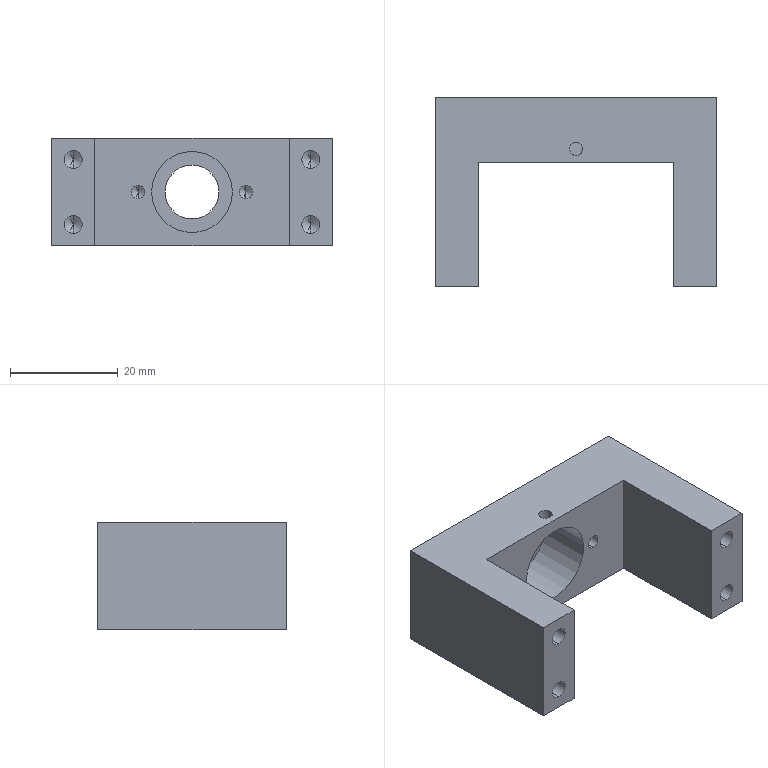Part | SolidWorks | features HoleWzd 3, ICE 3, Extrusion 1 | 1 solid | 41 faces | box 52 x 35 x 20 mm | volume 17449 mm3 | cylinder 18 | cone 12 | plane 11 | commonest cylinder face diameters 3.3 x8 2.5 x6 10 x2 15 x2
STEP:
#1=CARTESIAN_POINT('',(-10.,26.259,1.25));
#2=VERTEX_POINT('',#1);
#3=CARTESIAN_POINT('',(-10.,26.259,-1.25));
#4=VERTEX_POINT('',#3);
#5=CARTESIAN_POINT('',(-10.,26.259,0.));
#6=DIRECTION('',(0.,-1.,0.));
#7=DIRECTION('',(0.,0.,-1.));
#8=AXIS2_PLACEMENT_3D('',#5,#6,#7);
#9=CIRCLE('',#8,1.25);
#10=EDGE_CURVE('',#2,#4,#9,.T.);
#11=ORIENTED_EDGE('',*,*,#10,.F.);
#12=CARTESIAN_POINT('',(-10.,16.259,1.25));
#13=VERTEX_POINT('',#12);
#14=CARTESIAN_POINT('',(-10.,16.259,1.25));
#15=DIRECTION('',(0.,-1.,0.));
#16=VECTOR('',#15,1000.);
#17=LINE('',#14,#16);
#18=EDGE_CURVE('',#2,#13,#17,.T.);
#19=ORIENTED_EDGE('',*,*,#18,.T.);
#20=CARTESIAN_POINT('',(-10.,16.259,-1.25));
#21=VERTEX_POINT('',#20);
#22=CARTESIAN_POINT('',(-10.,16.259,0.));
#23=DIRECTION('',(0.,-1.,0.));
#24=DIRECTION('',(0.,0.,-1.));
#25=AXIS2_PLACEMENT_3D('',#22,#23,#24);
#26=CIRCLE('',#25,1.25);
#27=EDGE_CURVE('',#13,#21,#26,.T.);
#28=ORIENTED_EDGE('',*,*,#27,.T.);
#29=CARTESIAN_POINT('',(-10.,16.259,-1.25));
#30=DIRECTION('',(0.,-1.,0.));
#31=VECTOR('',#30,1000.);
#32=LINE('',#29,#31);
#33=EDGE_CURVE('',#4,#21,#32,.T.);
#34=ORIENTED_EDGE('',*,*,#33,.F.);
#35=EDGE_LOOP('',(#11,#19,#28,#34));
#36=FACE_OUTER_BOUND('',#35,.T.);
#37=CARTESIAN_POINT('',(-10.,16.259,0.));
#38=DIRECTION('',(0.,-1.,0.));
#39=DIRECTION('',(0.,0.,-1.));
#40=AXIS2_PLACEMENT_3D('',#37,#38,#39);
#41=CYLINDRICAL_SURFACE('',#40,1.25);
#42=ADVANCED_FACE('',(#36),#41,.F.);
#43=CARTESIAN_POINT('',(-10.,27.01,0.));
#44=VERTEX_POINT('',#43);
#45=CARTESIAN_POINT('',(-10.,26.259,-1.25));
#46=DIRECTION('',(0.,-0.515,-0.8572));
#47=VECTOR('',#46,1000.);
#48=LINE('',#45,#47);
#49=EDGE_CURVE('',#44,#4,#48,.T.);
#50=ORIENTED_EDGE('',*,*,#49,.F.);
#51=CARTESIAN_POINT('',(-10.,26.259,1.25));
#52=DIRECTION('',(0.,-0.515,0.8572));
#53=VECTOR('',#52,1000.);
#54=LINE('',#51,#53);
#55=EDGE_CURVE('',#44,#2,#54,.T.);
#56=ORIENTED_EDGE('',*,*,#55,.T.);
#57=ORIENTED_EDGE('',*,*,#10,.T.);
#58=EDGE_LOOP('',(#50,#56,#57));
#59=FACE_OUTER_BOUND('',#58,.T.);
#60=CARTESIAN_POINT('',(-10.,26.259,0.));
#61=DIRECTION('',(0.,-1.,0.));
#62=DIRECTION('',(0.,0.,-1.));
#63=AXIS2_PLACEMENT_3D('',#60,#61,#62);
#64=CONICAL_SURFACE('',#63,1.25,1.03);
#65=ADVANCED_FACE('',(#59),#64,.F.);
#66=CARTESIAN_POINT('',(10.,26.259,1.25));
#67=VERTEX_POINT('',#66);
#68=CARTESIAN_POINT('',(10.,26.259,-1.25));
#69=VERTEX_POINT('',#68);
#70=CARTESIAN_POINT('',(10.,26.259,0.));
#71=DIRECTION('',(0.,-1.,0.));
#72=DIRECTION('',(0.,0.,-1.));
#73=AXIS2_PLACEMENT_3D('',#70,#71,#72);
#74=CIRCLE('',#73,1.25);
#75=EDGE_CURVE('',#67,#69,#74,.T.);
#76=ORIENTED_EDGE('',*,*,#75,.F.);
#77=CARTESIAN_POINT('',(10.,16.259,1.25));
#78=VERTEX_POINT('',#77);
#79=CARTESIAN_POINT('',(10.,16.259,1.25));
#80=DIRECTION('',(0.,-1.,0.));
#81=VECTOR('',#80,1000.);
#82=LINE('',#79,#81);
#83=EDGE_CURVE('',#67,#78,#82,.T.);
#84=ORIENTED_EDGE('',*,*,#83,.T.);
#85=CARTESIAN_POINT('',(10.,16.259,-1.25));
#86=VERTEX_POINT('',#85);
#87=CARTESIAN_POINT('',(10.,16.259,0.));
#88=DIRECTION('',(0.,-1.,0.));
#89=DIRECTION('',(0.,0.,-1.));
#90=AXIS2_PLACEMENT_3D('',#87,#88,#89);
#91=CIRCLE('',#90,1.25);
#92=EDGE_CURVE('',#78,#86,#91,.T.);
#93=ORIENTED_EDGE('',*,*,#92,.T.);
#94=CARTESIAN_POINT('',(10.,16.259,-1.25));
#95=DIRECTION('',(0.,-1.,0.));
#96=VECTOR('',#95,1000.);
#97=LINE('',#94,#96);
#98=EDGE_CURVE('',#69,#86,#97,.T.);
#99=ORIENTED_EDGE('',*,*,#98,.F.);
#100=EDGE_LOOP('',(#76,#84,#93,#99));
#101=FACE_OUTER_BOUND('',#100,.T.);
#102=CARTESIAN_POINT('',(10.,16.259,0.));
#103=DIRECTION('',(0.,-1.,0.));
#104=DIRECTION('',(0.,0.,-1.));
#105=AXIS2_PLACEMENT_3D('',#102,#103,#104);
#106=CYLINDRICAL_SURFACE('',#105,1.25);
#107=ADVANCED_FACE('',(#101),#106,.F.);
#108=CARTESIAN_POINT('',(10.,27.01,0.));
#109=VERTEX_POINT('',#108);
#110=CARTESIAN_POINT('',(10.,26.259,-1.25));
#111=DIRECTION('',(0.,-0.515,-0.8572));
#112=VECTOR('',#111,1000.);
#113=LINE('',#110,#112);
#114=EDGE_CURVE('',#109,#69,#113,.T.);
#115=ORIENTED_EDGE('',*,*,#114,.F.);
#116=CARTESIAN_POINT('',(10.,26.259,1.25));
#117=DIRECTION('',(0.,-0.515,0.8572));
#118=VECTOR('',#117,1000.);
#119=LINE('',#116,#118);
#120=EDGE_CURVE('',#109,#67,#119,.T.);
#121=ORIENTED_EDGE('',*,*,#120,.T.);
#122=ORIENTED_EDGE('',*,*,#75,.T.);
#123=EDGE_LOOP('',(#115,#121,#122));
#124=FACE_OUTER_BOUND('',#123,.T.);
#125=CARTESIAN_POINT('',(10.,26.259,0.));
#126=DIRECTION('',(0.,-1.,0.));
#127=DIRECTION('',(0.,0.,-1.));
#128=AXIS2_PLACEMENT_3D('',#125,#126,#127);
#129=CONICAL_SURFACE('',#128,1.25,1.03);
#130=ADVANCED_FACE('',(#124),#129,.F.);
#131=CARTESIAN_POINT('',(-1.25,18.759,7.395));
#132=VERTEX_POINT('',#131);
#133=CARTESIAN_POINT('',(1.25,18.759,7.395));
#134=VERTEX_POINT('',#133);
#135=CARTESIAN_POINT('',(-1.25,18.759,7.395));
#136=CARTESIAN_POINT('',(-1.25,18.596,7.395));
#137=CARTESIAN_POINT('',(-1.217,18.431,7.401));
#138=CARTESIAN_POINT('',(-1.092,18.13,7.42));
#139=CARTESIAN_POINT('',(-0.9996,17.991,7.434));
#140=CARTESIAN_POINT('',(-0.8269,17.818,7.455));
#141=CARTESIAN_POINT('',(-0.7627,17.766,7.461));
#142=CARTESIAN_POINT('',(-0.6272,17.675,7.474));
#143=CARTESIAN_POINT('',(-0.5555,17.636,7.48));
#144=CARTESIAN_POINT('',(-0.3283,17.542,7.494));
#145=CARTESIAN_POINT('',(-0.1659,17.509,7.5));
#146=CARTESIAN_POINT('',(0.1644,17.509,7.5));
#147=CARTESIAN_POINT('',(0.3271,17.542,7.494));
#148=CARTESIAN_POINT('',(0.6295,17.667,7.475));
#149=CARTESIAN_POINT('',(0.7682,17.76,7.461));
#150=CARTESIAN_POINT('',(0.9984,17.99,7.434));
#151=CARTESIAN_POINT('',(1.092,18.129,7.42));
#152=CARTESIAN_POINT('',(1.217,18.429,7.401));
#153=CARTESIAN_POINT('',(1.25,18.594,7.395));
#154=CARTESIAN_POINT('',(1.25,18.759,7.395));
#155=B_SPLINE_CURVE_WITH_KNOTS('',3,(#135,#136,#137,#138,#139,#140,#141,#142,#143,#144,#145,#146,#147,#148,#149,#150,#151,#152,#153,#154),.UNSPECIFIED.,.F.,.F.,(4,2,2,2,2,2,2,2,2,4),(0.003915,0.004404,0.004893,0.005138,0.005383,0.005872,0.006361,0.00685,0.00734,0.007829),.UNSPECIFIED.);
#156=EDGE_CURVE('',#132,#134,#155,.T.);
#157=ORIENTED_EDGE('',*,*,#156,.F.);
#158=CARTESIAN_POINT('',(-1.25,18.759,10.));
#159=VERTEX_POINT('',#158);
#160=CARTESIAN_POINT('',(-1.25,18.759,10.));
#161=DIRECTION('',(0.,0.,1.));
#162=VECTOR('',#161,1000.);
#163=LINE('',#160,#162);
#164=EDGE_CURVE('',#132,#159,#163,.T.);
#165=ORIENTED_EDGE('',*,*,#164,.T.);
#166=CARTESIAN_POINT('',(1.25,18.759,10.));
#167=VERTEX_POINT('',#166);
#168=CARTESIAN_POINT('',(0.,18.759,10.));
#169=DIRECTION('',(0.,0.,1.));
#170=DIRECTION('',(1.,0.,0.));
#171=AXIS2_PLACEMENT_3D('',#168,#169,#170);
#172=CIRCLE('',#171,1.25);
#173=EDGE_CURVE('',#159,#167,#172,.T.);
#174=ORIENTED_EDGE('',*,*,#173,.T.);
#175=CARTESIAN_POINT('',(1.25,18.759,10.));
#176=DIRECTION('',(0.,0.,1.));
#177=VECTOR('',#176,1000.);
#178=LINE('',#175,#177);
#179=EDGE_CURVE('',#134,#167,#178,.T.);
#180=ORIENTED_EDGE('',*,*,#179,.F.);
#181=EDGE_LOOP('',(#157,#165,#174,#180));
#182=FACE_OUTER_BOUND('',#181,.T.);
#183=CARTESIAN_POINT('',(0.,18.759,10.));
#184=DIRECTION('',(0.,0.,1.));
#185=DIRECTION('',(1.,0.,0.));
#186=AXIS2_PLACEMENT_3D('',#183,#184,#185);
#187=CYLINDRICAL_SURFACE('',#186,1.25);
#188=ADVANCED_FACE('',(#182),#187,.F.);
#189=CARTESIAN_POINT('',(-7.5,26.259,0.));
#190=VERTEX_POINT('',#189);
#191=CARTESIAN_POINT('',(7.5,26.259,0.));
#192=VERTEX_POINT('',#191);
#193=CARTESIAN_POINT('',(0.,26.259,0.));
#194=DIRECTION('',(0.,-1.,0.));
#195=DIRECTION('',(1.,0.,0.));
#196=AXIS2_PLACEMENT_3D('',#193,#194,#195);
#197=CIRCLE('',#196,7.5);
#198=EDGE_CURVE('',#190,#192,#197,.T.);
#199=ORIENTED_EDGE('',*,*,#198,.F.);
#200=CARTESIAN_POINT('',(-7.5,16.259,0.));
#201=VERTEX_POINT('',#200);
#202=CARTESIAN_POINT('',(-7.5,26.259,0.));
#203=DIRECTION('',(0.,-1.,0.));
#204=VECTOR('',#203,1000.);
#205=LINE('',#202,#204);
#206=EDGE_CURVE('',#190,#201,#205,.T.);
#207=ORIENTED_EDGE('',*,*,#206,.T.);
#208=CARTESIAN_POINT('',(7.5,16.259,0.));
#209=VERTEX_POINT('',#208);
#210=CARTESIAN_POINT('',(0.,16.259,0.));
#211=DIRECTION('',(0.,-1.,0.));
#212=DIRECTION('',(1.,0.,0.));
#213=AXIS2_PLACEMENT_3D('',#210,#211,#212);
#214=CIRCLE('',#213,7.5);
#215=EDGE_CURVE('',#201,#209,#214,.T.);
#216=ORIENTED_EDGE('',*,*,#215,.T.);
#217=CARTESIAN_POINT('',(7.5,26.259,0.));
#218=DIRECTION('',(0.,-1.,0.));
#219=VECTOR('',#218,1000.);
#220=LINE('',#217,#219);
#221=EDGE_CURVE('',#192,#209,#220,.T.);
#222=ORIENTED_EDGE('',*,*,#221,.F.);
#223=EDGE_LOOP('',(#199,#207,#216,#222));
#224=FACE_OUTER_BOUND('',#223,.T.);
#225=CARTESIAN_POINT('',(0.,26.259,0.));
#226=DIRECTION('',(0.,-1.,0.));
#227=DIRECTION('',(1.,0.,0.));
#228=AXIS2_PLACEMENT_3D('',#225,#226,#227);
#229=CYLINDRICAL_SURFACE('',#228,7.5);
#230=ADVANCED_FACE('',(#224),#229,.F.);
#231=CARTESIAN_POINT('',(22.,3.259,-4.35));
#232=VERTEX_POINT('',#231);
#233=CARTESIAN_POINT('',(22.,3.259,-7.65));
#234=VERTEX_POINT('',#233);
#235=CARTESIAN_POINT('',(22.,3.259,-6.));
#236=DIRECTION('',(0.,-1.,0.));
#237=DIRECTION('',(0.,0.,-1.));
#238=AXIS2_PLACEMENT_3D('',#235,#236,#237);
#239=CIRCLE('',#238,1.65);
#240=EDGE_CURVE('',#232,#234,#239,.T.);
#241=ORIENTED_EDGE('',*,*,#240,.F.);
#242=CARTESIAN_POINT('',(22.,-6.741,-4.35));
#243=VERTEX_POINT('',#242);
#244=CARTESIAN_POINT('',(22.,-6.741,-4.35));
#245=DIRECTION('',(0.,-1.,0.));
#246=VECTOR('',#245,1000.);
#247=LINE('',#244,#246);
#248=EDGE_CURVE('',#232,#243,#247,.T.);
#249=ORIENTED_EDGE('',*,*,#248,.T.);
#250=CARTESIAN_POINT('',(22.,-6.741,-7.65));
#251=VERTEX_POINT('',#250);
#252=CARTESIAN_POINT('',(22.,-6.741,-6.));
#253=DIRECTION('',(0.,-1.,0.));
#254=DIRECTION('',(0.,0.,-1.));
#255=AXIS2_PLACEMENT_3D('',#252,#253,#254);
#256=CIRCLE('',#255,1.65);
#257=EDGE_CURVE('',#243,#251,#256,.T.);
#258=ORIENTED_EDGE('',*,*,#257,.T.);
#259=CARTESIAN_POINT('',(22.,-6.741,-7.65));
#260=DIRECTION('',(0.,-1.,0.));
#261=VECTOR('',#260,1000.);
#262=LINE('',#259,#261);
#263=EDGE_CURVE('',#234,#251,#262,.T.);
#264=ORIENTED_EDGE('',*,*,#263,.F.);
#265=EDGE_LOOP('',(#241,#249,#258,#264));
#266=FACE_OUTER_BOUND('',#265,.T.);
#267=CARTESIAN_POINT('',(22.,-6.741,-6.));
#268=DIRECTION('',(0.,-1.,0.));
#269=DIRECTION('',(0.,0.,-1.));
#270=AXIS2_PLACEMENT_3D('',#267,#268,#269);
#271=CYLINDRICAL_SURFACE('',#270,1.65);
#272=ADVANCED_FACE('',(#266),#271,.F.);
#273=CARTESIAN_POINT('',(22.,4.251,-6.));
#274=VERTEX_POINT('',#273);
#275=CARTESIAN_POINT('',(22.,3.259,-7.65));
#276=DIRECTION('',(0.,-0.515,-0.8572));
#277=VECTOR('',#276,1000.);
#278=LINE('',#275,#277);
#279=EDGE_CURVE('',#274,#234,#278,.T.);
#280=ORIENTED_EDGE('',*,*,#279,.F.);
#281=CARTESIAN_POINT('',(22.,3.259,-4.35));
#282=DIRECTION('',(0.,-0.515,0.8572));
#283=VECTOR('',#282,1000.);
#284=LINE('',#281,#283);
#285=EDGE_CURVE('',#274,#232,#284,.T.);
#286=ORIENTED_EDGE('',*,*,#285,.T.);
#287=ORIENTED_EDGE('',*,*,#240,.T.);
#288=EDGE_LOOP('',(#280,#286,#287));
#289=FACE_OUTER_BOUND('',#288,.T.);
#290=CARTESIAN_POINT('',(22.,3.259,-6.));
#291=DIRECTION('',(0.,-1.,0.));
#292=DIRECTION('',(0.,0.,-1.));
#293=AXIS2_PLACEMENT_3D('',#290,#291,#292);
#294=CONICAL_SURFACE('',#293,1.65,1.03);
#295=ADVANCED_FACE('',(#289),#294,.F.);
#296=CARTESIAN_POINT('',(22.,3.259,7.65));
#297=VERTEX_POINT('',#296);
#298=CARTESIAN_POINT('',(22.,3.259,4.35));
#299=VERTEX_POINT('',#298);
#300=CARTESIAN_POINT('',(22.,3.259,6.));
#301=DIRECTION('',(0.,-1.,0.));
#302=DIRECTION('',(0.,0.,-1.));
#303=AXIS2_PLACEMENT_3D('',#300,#301,#302);
#304=CIRCLE('',#303,1.65);
#305=EDGE_CURVE('',#297,#299,#304,.T.);
#306=ORIENTED_EDGE('',*,*,#305,.F.);
#307=CARTESIAN_POINT('',(22.,-6.741,7.65));
#308=VERTEX_POINT('',#307);
#309=CARTESIAN_POINT('',(22.,-6.741,7.65));
#310=DIRECTION('',(0.,-1.,0.));
#311=VECTOR('',#310,1000.);
#312=LINE('',#309,#311);
#313=EDGE_CURVE('',#297,#308,#312,.T.);
#314=ORIENTED_EDGE('',*,*,#313,.T.);
#315=CARTESIAN_POINT('',(22.,-6.741,4.35));
#316=VERTEX_POINT('',#315);
#317=CARTESIAN_POINT('',(22.,-6.741,6.));
#318=DIRECTION('',(0.,-1.,0.));
#319=DIRECTION('',(0.,0.,-1.));
#320=AXIS2_PLACEMENT_3D('',#317,#318,#319);
#321=CIRCLE('',#320,1.65);
#322=EDGE_CURVE('',#308,#316,#321,.T.);
#323=ORIENTED_EDGE('',*,*,#322,.T.);
#324=CARTESIAN_POINT('',(22.,-6.741,4.35));
#325=DIRECTION('',(0.,-1.,0.));
#326=VECTOR('',#325,1000.);
#327=LINE('',#324,#326);
#328=EDGE_CURVE('',#299,#316,#327,.T.);
#329=ORIENTED_EDGE('',*,*,#328,.F.);
#330=EDGE_LOOP('',(#306,#314,#323,#329));
#331=FACE_OUTER_BOUND('',#330,.T.);
#332=CARTESIAN_POINT('',(22.,-6.741,6.));
#333=DIRECTION('',(0.,-1.,0.));
#334=DIRECTION('',(0.,0.,-1.));
#335=AXIS2_PLACEMENT_3D('',#332,#333,#334);
#336=CYLINDRICAL_SURFACE('',#335,1.65);
#337=ADVANCED_FACE('',(#331),#336,.F.);
#338=CARTESIAN_POINT('',(22.,4.251,6.));
#339=VERTEX_POINT('',#338);
#340=CARTESIAN_POINT('',(22.,3.259,4.35));
#341=DIRECTION('',(0.,-0.515,-0.8572));
#342=VECTOR('',#341,1000.);
#343=LINE('',#340,#342);
#344=EDGE_CURVE('',#339,#299,#343,.T.);
#345=ORIENTED_EDGE('',*,*,#344,.F.);
#346=CARTESIAN_POINT('',(22.,3.259,7.65));
#347=DIRECTION('',(0.,-0.515,0.8572));
#348=VECTOR('',#347,1000.);
#349=LINE('',#346,#348);
#350=EDGE_CURVE('',#339,#297,#349,.T.);
#351=ORIENTED_EDGE('',*,*,#350,.T.);
#352=ORIENTED_EDGE('',*,*,#305,.T.);
#353=EDGE_LOOP('',(#345,#351,#352));
#354=FACE_OUTER_BOUND('',#353,.T.);
#355=CARTESIAN_POINT('',(22.,3.259,6.));
#356=DIRECTION('',(0.,-1.,0.));
#357=DIRECTION('',(0.,0.,-1.));
#358=AXIS2_PLACEMENT_3D('',#355,#356,#357);
#359=CONICAL_SURFACE('',#358,1.65,1.03);
#360=ADVANCED_FACE('',(#354),#359,.F.);
#361=CARTESIAN_POINT('',(-22.,3.259,-4.35));
#362=VERTEX_POINT('',#361);
#363=CARTESIAN_POINT('',(-22.,3.259,-7.65));
#364=VERTEX_POINT('',#363);
#365=CARTESIAN_POINT('',(-22.,3.259,-6.));
#366=DIRECTION('',(0.,-1.,0.));
#367=DIRECTION('',(0.,0.,-1.));
#368=AXIS2_PLACEMENT_3D('',#365,#366,#367);
#369=CIRCLE('',#368,1.65);
#370=EDGE_CURVE('',#362,#364,#369,.T.);
#371=ORIENTED_EDGE('',*,*,#370,.F.);
#372=CARTESIAN_POINT('',(-22.,-6.741,-4.35));
#373=VERTEX_POINT('',#372);
#374=CARTESIAN_POINT('',(-22.,-6.741,-4.35));
#375=DIRECTION('',(0.,-1.,0.));
#376=VECTOR('',#375,1000.);
#377=LINE('',#374,#376);
#378=EDGE_CURVE('',#362,#373,#377,.T.);
#379=ORIENTED_EDGE('',*,*,#378,.T.);
#380=CARTESIAN_POINT('',(-22.,-6.741,-7.65));
#381=VERTEX_POINT('',#380);
#382=CARTESIAN_POINT('',(-22.,-6.741,-6.));
#383=DIRECTION('',(0.,-1.,0.));
#384=DIRECTION('',(0.,0.,-1.));
#385=AXIS2_PLACEMENT_3D('',#382,#383,#384);
#386=CIRCLE('',#385,1.65);
#387=EDGE_CURVE('',#373,#381,#386,.T.);
#388=ORIENTED_EDGE('',*,*,#387,.T.);
#389=CARTESIAN_POINT('',(-22.,-6.741,-7.65));
#390=DIRECTION('',(0.,-1.,0.));
#391=VECTOR('',#390,1000.);
#392=LINE('',#389,#391);
#393=EDGE_CURVE('',#364,#381,#392,.T.);
#394=ORIENTED_EDGE('',*,*,#393,.F.);
#395=EDGE_LOOP('',(#371,#379,#388,#394));
#396=FACE_OUTER_BOUND('',#395,.T.);
#397=CARTESIAN_POINT('',(-22.,-6.741,-6.));
#398=DIRECTION('',(0.,-1.,0.));
#399=DIRECTION('',(0.,0.,-1.));
#400=AXIS2_PLACEMENT_3D('',#397,#398,#399);
#401=CYLINDRICAL_SURFACE('',#400,1.65);
#402=ADVANCED_FACE('',(#396),#401,.F.);
#403=CARTESIAN_POINT('',(-22.,4.251,-6.));
#404=VERTEX_POINT('',#403);
#405=CARTESIAN_POINT('',(-22.,3.259,-7.65));
#406=DIRECTION('',(0.,-0.515,-0.8572));
#407=VECTOR('',#406,1000.);
#408=LINE('',#405,#407);
#409=EDGE_CURVE('',#404,#364,#408,.T.);
#410=ORIENTED_EDGE('',*,*,#409,.F.);
#411=CARTESIAN_POINT('',(-22.,3.259,-4.35));
#412=DIRECTION('',(0.,-0.515,0.8572));
#413=VECTOR('',#412,1000.);
#414=LINE('',#411,#413);
#415=EDGE_CURVE('',#404,#362,#414,.T.);
#416=ORIENTED_EDGE('',*,*,#415,.T.);
#417=ORIENTED_EDGE('',*,*,#370,.T.);
#418=EDGE_LOOP('',(#410,#416,#417));
#419=FACE_OUTER_BOUND('',#418,.T.);
#420=CARTESIAN_POINT('',(-22.,3.259,-6.));
#421=DIRECTION('',(0.,-1.,0.));
#422=DIRECTION('',(0.,0.,-1.));
#423=AXIS2_PLACEMENT_3D('',#420,#421,#422);
#424=CONICAL_SURFACE('',#423,1.65,1.03);
#425=ADVANCED_FACE('',(#419),#424,.F.);
#426=CARTESIAN_POINT('',(-22.,3.259,7.65));
#427=VERTEX_POINT('',#426);
#428=CARTESIAN_POINT('',(-22.,3.259,4.35));
#429=VERTEX_POINT('',#428);
#430=CARTESIAN_POINT('',(-22.,3.259,6.));
#431=DIRECTION('',(0.,-1.,0.));
#432=DIRECTION('',(0.,0.,-1.));
#433=AXIS2_PLACEMENT_3D('',#430,#431,#432);
#434=CIRCLE('',#433,1.65);
#435=EDGE_CURVE('',#427,#429,#434,.T.);
#436=ORIENTED_EDGE('',*,*,#435,.F.);
#437=CARTESIAN_POINT('',(-22.,-6.741,7.65));
#438=VERTEX_POINT('',#437);
#439=CARTESIAN_POINT('',(-22.,-6.741,7.65));
#440=DIRECTION('',(0.,-1.,0.));
#441=VECTOR('',#440,1000.);
#442=LINE('',#439,#441);
#443=EDGE_CURVE('',#427,#438,#442,.T.);
#444=ORIENTED_EDGE('',*,*,#443,.T.);
#445=CARTESIAN_POINT('',(-22.,-6.741,4.35));
#446=VERTEX_POINT('',#445);
#447=CARTESIAN_POINT('',(-22.,-6.741,6.));
#448=DIRECTION('',(0.,-1.,0.));
#449=DIRECTION('',(0.,0.,-1.));
#450=AXIS2_PLACEMENT_3D('',#447,#448,#449);
#451=CIRCLE('',#450,1.65);
#452=EDGE_CURVE('',#438,#446,#451,.T.);
#453=ORIENTED_EDGE('',*,*,#452,.T.);
#454=CARTESIAN_POINT('',(-22.,-6.741,4.35));
#455=DIRECTION('',(0.,-1.,0.));
#456=VECTOR('',#455,1000.);
#457=LINE('',#454,#456);
#458=EDGE_CURVE('',#429,#446,#457,.T.);
#459=ORIENTED_EDGE('',*,*,#458,.F.);
#460=EDGE_LOOP('',(#436,#444,#453,#459));
#461=FACE_OUTER_BOUND('',#460,.T.);
#462=CARTESIAN_POINT('',(-22.,-6.741,6.));
#463=DIRECTION('',(0.,-1.,0.));
#464=DIRECTION('',(0.,0.,-1.));
#465=AXIS2_PLACEMENT_3D('',#462,#463,#464);
#466=CYLINDRICAL_SURFACE('',#465,1.65);
#467=ADVANCED_FACE('',(#461),#466,.F.);
#468=CARTESIAN_POINT('',(-22.,4.251,6.));
#469=VERTEX_POINT('',#468);
#470=CARTESIAN_POINT('',(-22.,3.259,4.35));
#471=DIRECTION('',(0.,-0.515,-0.8572));
#472=VECTOR('',#471,1000.);
#473=LINE('',#470,#472);
#474=EDGE_CURVE('',#469,#429,#473,.T.);
#475=ORIENTED_EDGE('',*,*,#474,.F.);
#476=CARTESIAN_POINT('',(-22.,3.259,7.65));
#477=DIRECTION('',(0.,-0.515,0.8572));
#478=VECTOR('',#477,1000.);
#479=LINE('',#476,#478);
#480=EDGE_CURVE('',#469,#427,#479,.T.);
#481=ORIENTED_EDGE('',*,*,#480,.T.);
#482=ORIENTED_EDGE('',*,*,#435,.T.);
#483=EDGE_LOOP('',(#475,#481,#482));
#484=FACE_OUTER_BOUND('',#483,.T.);
#485=CARTESIAN_POINT('',(-22.,3.259,6.));
#486=DIRECTION('',(0.,-1.,0.));
#487=DIRECTION('',(0.,0.,-1.));
#488=AXIS2_PLACEMENT_3D('',#485,#486,#487);
#489=CONICAL_SURFACE('',#488,1.65,1.03);
#490=ADVANCED_FACE('',(#484),#489,.F.);
#491=CARTESIAN_POINT('',(5.,26.259,0.));
#492=VERTEX_POINT('',#491);
#493=CARTESIAN_POINT('',(-5.,26.259,0.));
#494=VERTEX_POINT('',#493);
#495=CARTESIAN_POINT('',(0.,26.259,0.));
#496=DIRECTION('',(0.,1.,0.));
#497=DIRECTION('',(1.,0.,0.));
#498=AXIS2_PLACEMENT_3D('',#495,#496,#497);
#499=CIRCLE('',#498,5.);
#500=EDGE_CURVE('',#492,#494,#499,.T.);
#501=ORIENTED_EDGE('',*,*,#500,.F.);
#502=CARTESIAN_POINT('',(5.,28.259,0.));
#503=VERTEX_POINT('',#502);
#504=CARTESIAN_POINT('',(5.,1.259,0.));
#505=DIRECTION('',(0.,1.,0.));
#506=VECTOR('',#505,1000.);
#507=LINE('',#504,#506);
#508=EDGE_CURVE('',#492,#503,#507,.T.);
#509=ORIENTED_EDGE('',*,*,#508,.T.);
#510=CARTESIAN_POINT('',(-5.,28.259,0.));
#511=VERTEX_POINT('',#510);
#512=CARTESIAN_POINT('',(0.,28.259,0.));
#513=DIRECTION('',(0.,1.,0.));
#514=DIRECTION('',(-1.,0.,0.));
#515=AXIS2_PLACEMENT_3D('',#512,#513,#514);
#516=CIRCLE('',#515,5.);
#517=EDGE_CURVE('',#503,#511,#516,.T.);
#518=ORIENTED_EDGE('',*,*,#517,.T.);
#519=CARTESIAN_POINT('',(-5.,1.259,0.));
#520=DIRECTION('',(0.,1.,0.));
#521=VECTOR('',#520,1000.);
#522=LINE('',#519,#521);
#523=EDGE_CURVE('',#494,#511,#522,.T.);
#524=ORIENTED_EDGE('',*,*,#523,.F.);
#525=EDGE_LOOP('',(#501,#509,#518,#524));
#526=FACE_OUTER_BOUND('',#525,.T.);
#527=CARTESIAN_POINT('',(0.,1.259,0.));
#528=DIRECTION('',(0.,1.,0.));
#529=DIRECTION('',(-1.,0.,0.));
#530=AXIS2_PLACEMENT_3D('',#527,#528,#529);
#531=CYLINDRICAL_SURFACE('',#530,5.);
#532=ADVANCED_FACE('',(#526),#531,.F.);
#533=ORIENTED_EDGE('',*,*,#508,.F.);
#534=CARTESIAN_POINT('',(0.,26.259,0.));
#535=DIRECTION('',(0.,1.,0.));
#536=DIRECTION('',(1.,0.,0.));
#537=AXIS2_PLACEMENT_3D('',#534,#535,#536);
#538=CIRCLE('',#537,5.);
#539=EDGE_CURVE('',#494,#492,#538,.T.);
#540=ORIENTED_EDGE('',*,*,#539,.F.);
#541=ORIENTED_EDGE('',*,*,#523,.T.);
#542=CARTESIAN_POINT('',(0.,28.259,0.));
#543=DIRECTION('',(0.,1.,0.));
#544=DIRECTION('',(-1.,0.,0.));
#545=AXIS2_PLACEMENT_3D('',#542,#543,#544);
#546=CIRCLE('',#545,5.);
#547=EDGE_CURVE('',#511,#503,#546,.T.);
#548=ORIENTED_EDGE('',*,*,#547,.T.);
#549=EDGE_LOOP('',(#533,#540,#541,#548));
#550=FACE_OUTER_BOUND('',#549,.T.);
#551=CARTESIAN_POINT('',(0.,1.259,0.));
#552=DIRECTION('',(0.,1.,0.));
#553=DIRECTION('',(-1.,0.,0.));
#554=AXIS2_PLACEMENT_3D('',#551,#552,#553);
#555=CYLINDRICAL_SURFACE('',#554,5.);
#556=ADVANCED_FACE('',(#550),#555,.F.);
#557=CARTESIAN_POINT('',(-26.,-6.741,-10.));
#558=VERTEX_POINT('',#557);
#559=CARTESIAN_POINT('',(-18.,-6.741,-10.));
#560=VERTEX_POINT('',#559);
#561=CARTESIAN_POINT('',(-18.,-6.741,-10.));
#562=DIRECTION('',(1.,0.,0.));
#563=VECTOR('',#562,1000.);
#564=LINE('',#561,#563);
#565=EDGE_CURVE('',#558,#560,#564,.T.);
#566=ORIENTED_EDGE('',*,*,#565,.T.);
#567=CARTESIAN_POINT('',(-18.,-6.741,10.));
#568=VERTEX_POINT('',#567);
#569=CARTESIAN_POINT('',(-18.,-6.741,10.));
#570=DIRECTION('',(0.,0.,-1.));
#571=VECTOR('',#570,1000.);
#572=LINE('',#569,#571);
#573=EDGE_CURVE('',#568,#560,#572,.T.);
#574=ORIENTED_EDGE('',*,*,#573,.F.);
#575=CARTESIAN_POINT('',(-26.,-6.741,10.));
#576=VERTEX_POINT('',#575);
#577=CARTESIAN_POINT('',(-18.,-6.741,10.));
#578=DIRECTION('',(1.,0.,0.));
#579=VECTOR('',#578,1000.);
#580=LINE('',#577,#579);
#581=EDGE_CURVE('',#576,#568,#580,.T.);
#582=ORIENTED_EDGE('',*,*,#581,.F.);
#583=CARTESIAN_POINT('',(-26.,-6.741,10.));
#584=DIRECTION('',(0.,0.,-1.));
#585=VECTOR('',#584,1000.);
#586=LINE('',#583,#585);
#587=EDGE_CURVE('',#576,#558,#586,.T.);
#588=ORIENTED_EDGE('',*,*,#587,.T.);
#589=EDGE_LOOP('',(#566,#574,#582,#588));
#590=FACE_OUTER_BOUND('',#589,.T.);
#591=CARTESIAN_POINT('',(-22.,-6.741,6.));
#592=DIRECTION('',(0.,-1.,0.));
#593=DIRECTION('',(0.,0.,-1.));
#594=AXIS2_PLACEMENT_3D('',#591,#592,#593);
#595=CIRCLE('',#594,1.65);
#596=EDGE_CURVE('',#446,#438,#595,.T.);
#597=ORIENTED_EDGE('',*,*,#596,.F.);
#598=ORIENTED_EDGE('',*,*,#452,.F.);
#599=EDGE_LOOP('',(#597,#598));
#600=FACE_BOUND('',#599,.T.);
#601=CARTESIAN_POINT('',(-22.,-6.741,-6.));
#602=DIRECTION('',(0.,-1.,0.));
#603=DIRECTION('',(0.,0.,-1.));
#604=AXIS2_PLACEMENT_3D('',#601,#602,#603);
#605=CIRCLE('',#604,1.65);
#606=EDGE_CURVE('',#381,#373,#605,.T.);
#607=ORIENTED_EDGE('',*,*,#606,.F.);
#608=ORIENTED_EDGE('',*,*,#387,.F.);
#609=EDGE_LOOP('',(#607,#608));
#610=FACE_BOUND('',#609,.T.);
#611=CARTESIAN_POINT('',(-18.,-6.741,10.));
#612=DIRECTION('',(0.,1.,0.));
#613=DIRECTION('',(-1.,0.,0.));
#614=AXIS2_PLACEMENT_3D('',#611,#612,#613);
#615=PLANE('',#614);
#616=ADVANCED_FACE('',(#590,#600,#610),#615,.F.);
#617=CARTESIAN_POINT('',(-18.,16.259,-10.));
#618=VERTEX_POINT('',#617);
#619=CARTESIAN_POINT('',(-18.,-6.741,-10.));
#620=DIRECTION('',(0.,1.,0.));
#621=VECTOR('',#620,1000.);
#622=LINE('',#619,#621);
#623=EDGE_CURVE('',#560,#618,#622,.T.);
#624=ORIENTED_EDGE('',*,*,#623,.T.);
#625=CARTESIAN_POINT('',(-18.,16.259,10.));
#626=VERTEX_POINT('',#625);
#627=CARTESIAN_POINT('',(-18.,16.259,10.));
#628=DIRECTION('',(0.,0.,-1.));
#629=VECTOR('',#628,1000.);
#630=LINE('',#627,#629);
#631=EDGE_CURVE('',#626,#618,#630,.T.);
#632=ORIENTED_EDGE('',*,*,#631,.F.);
#633=CARTESIAN_POINT('',(-18.,-6.741,10.));
#634=DIRECTION('',(0.,1.,0.));
#635=VECTOR('',#634,1000.);
#636=LINE('',#633,#635);
#637=EDGE_CURVE('',#568,#626,#636,.T.);
#638=ORIENTED_EDGE('',*,*,#637,.F.);
#639=ORIENTED_EDGE('',*,*,#573,.T.);
#640=EDGE_LOOP('',(#624,#632,#638,#639));
#641=FACE_OUTER_BOUND('',#640,.T.);
#642=CARTESIAN_POINT('',(-18.,-6.741,10.));
#643=DIRECTION('',(-1.,0.,0.));
#644=DIRECTION('',(0.,0.,1.));
#645=AXIS2_PLACEMENT_3D('',#642,#643,#644);
#646=PLANE('',#645);
#647=ADVANCED_FACE('',(#641),#646,.F.);
#648=CARTESIAN_POINT('',(-10.,16.259,0.));
#649=DIRECTION('',(0.,-1.,0.));
#650=DIRECTION('',(0.,0.,-1.));
#651=AXIS2_PLACEMENT_3D('',#648,#649,#650);
#652=CIRCLE('',#651,1.25);
#653=EDGE_CURVE('',#21,#13,#652,.T.);
#654=ORIENTED_EDGE('',*,*,#653,.F.);
#655=ORIENTED_EDGE('',*,*,#27,.F.);
#656=EDGE_LOOP('',(#654,#655));
#657=FACE_BOUND('',#656,.T.);
#658=CARTESIAN_POINT('',(10.,16.259,0.));
#659=DIRECTION('',(0.,-1.,0.));
#660=DIRECTION('',(0.,0.,-1.));
#661=AXIS2_PLACEMENT_3D('',#658,#659,#660);
#662=CIRCLE('',#661,1.25);
#663=EDGE_CURVE('',#86,#78,#662,.T.);
#664=ORIENTED_EDGE('',*,*,#663,.F.);
#665=ORIENTED_EDGE('',*,*,#92,.F.);
#666=EDGE_LOOP('',(#664,#665));
#667=FACE_BOUND('',#666,.T.);
#668=CARTESIAN_POINT('',(0.,16.259,0.));
#669=DIRECTION('',(0.,-1.,0.));
#670=DIRECTION('',(1.,0.,0.));
#671=AXIS2_PLACEMENT_3D('',#668,#669,#670);
#672=CIRCLE('',#671,7.5);
#673=EDGE_CURVE('',#209,#201,#672,.T.);
#674=ORIENTED_EDGE('',*,*,#673,.F.);
#675=ORIENTED_EDGE('',*,*,#215,.F.);
#676=EDGE_LOOP('',(#674,#675));
#677=FACE_BOUND('',#676,.T.);
#678=CARTESIAN_POINT('',(18.,16.259,-10.));
#679=VERTEX_POINT('',#678);
#680=CARTESIAN_POINT('',(-18.,16.259,-10.));
#681=DIRECTION('',(1.,0.,0.));
#682=VECTOR('',#681,1000.);
#683=LINE('',#680,#682);
#684=EDGE_CURVE('',#618,#679,#683,.T.);
#685=ORIENTED_EDGE('',*,*,#684,.T.);
#686=CARTESIAN_POINT('',(18.,16.259,10.));
#687=VERTEX_POINT('',#686);
#688=CARTESIAN_POINT('',(18.,16.259,10.));
#689=DIRECTION('',(0.,0.,-1.));
#690=VECTOR('',#689,1000.);
#691=LINE('',#688,#690);
#692=EDGE_CURVE('',#687,#679,#691,.T.);
#693=ORIENTED_EDGE('',*,*,#692,.F.);
#694=CARTESIAN_POINT('',(-18.,16.259,10.));
#695=DIRECTION('',(1.,0.,0.));
#696=VECTOR('',#695,1000.);
#697=LINE('',#694,#696);
#698=EDGE_CURVE('',#626,#687,#697,.T.);
#699=ORIENTED_EDGE('',*,*,#698,.F.);
#700=ORIENTED_EDGE('',*,*,#631,.T.);
#701=EDGE_LOOP('',(#685,#693,#699,#700));
#702=FACE_OUTER_BOUND('',#701,.T.);
#703=CARTESIAN_POINT('',(-18.,16.259,10.));
#704=DIRECTION('',(0.,1.,0.));
#705=DIRECTION('',(-1.,0.,0.));
#706=AXIS2_PLACEMENT_3D('',#703,#704,#705);
#707=PLANE('',#706);
#708=ADVANCED_FACE('',(#657,#667,#677,#702),#707,.F.);
#709=CARTESIAN_POINT('',(18.,-6.741,-10.));
#710=VERTEX_POINT('',#709);
#711=CARTESIAN_POINT('',(18.,-6.741,-10.));
#712=DIRECTION('',(0.,-1.,0.));
#713=VECTOR('',#712,1000.);
#714=LINE('',#711,#713);
#715=EDGE_CURVE('',#679,#710,#714,.T.);
#716=ORIENTED_EDGE('',*,*,#715,.T.);
#717=CARTESIAN_POINT('',(18.,-6.741,10.));
#718=VERTEX_POINT('',#717);
#719=CARTESIAN_POINT('',(18.,-6.741,10.));
#720=DIRECTION('',(0.,0.,-1.));
#721=VECTOR('',#720,1000.);
#722=LINE('',#719,#721);
#723=EDGE_CURVE('',#718,#710,#722,.T.);
#724=ORIENTED_EDGE('',*,*,#723,.F.);
#725=CARTESIAN_POINT('',(18.,-6.741,10.));
#726=DIRECTION('',(0.,-1.,0.));
#727=VECTOR('',#726,1000.);
#728=LINE('',#725,#727);
#729=EDGE_CURVE('',#687,#718,#728,.T.);
#730=ORIENTED_EDGE('',*,*,#729,.F.);
#731=ORIENTED_EDGE('',*,*,#692,.T.);
#732=EDGE_LOOP('',(#716,#724,#730,#731));
#733=FACE_OUTER_BOUND('',#732,.T.);
#734=CARTESIAN_POINT('',(18.,-6.741,10.));
#735=DIRECTION('',(1.,0.,0.));
#736=DIRECTION('',(0.,1.,0.));
#737=AXIS2_PLACEMENT_3D('',#734,#735,#736);
#738=PLANE('',#737);
#739=ADVANCED_FACE('',(#733),#738,.F.);
#740=CARTESIAN_POINT('',(22.,-6.741,-6.));
#741=DIRECTION('',(0.,-1.,0.));
#742=DIRECTION('',(0.,0.,-1.));
#743=AXIS2_PLACEMENT_3D('',#740,#741,#742);
#744=CIRCLE('',#743,1.65);
#745=EDGE_CURVE('',#251,#243,#744,.T.);
#746=ORIENTED_EDGE('',*,*,#745,.F.);
#747=ORIENTED_EDGE('',*,*,#257,.F.);
#748=EDGE_LOOP('',(#746,#747));
#749=FACE_BOUND('',#748,.T.);
#750=CARTESIAN_POINT('',(22.,-6.741,6.));
#751=DIRECTION('',(0.,-1.,0.));
#752=DIRECTION('',(0.,0.,-1.));
#753=AXIS2_PLACEMENT_3D('',#750,#751,#752);
#754=CIRCLE('',#753,1.65);
#755=EDGE_CURVE('',#316,#308,#754,.T.);
#756=ORIENTED_EDGE('',*,*,#755,.F.);
#757=ORIENTED_EDGE('',*,*,#322,.F.);
#758=EDGE_LOOP('',(#756,#757));
#759=FACE_BOUND('',#758,.T.);
#760=CARTESIAN_POINT('',(26.,-6.741,-10.));
#761=VERTEX_POINT('',#760);
#762=CARTESIAN_POINT('',(18.,-6.741,-10.));
#763=DIRECTION('',(1.,0.,0.));
#764=VECTOR('',#763,1000.);
#765=LINE('',#762,#764);
#766=EDGE_CURVE('',#710,#761,#765,.T.);
#767=ORIENTED_EDGE('',*,*,#766,.T.);
#768=CARTESIAN_POINT('',(26.,-6.741,10.));
#769=VERTEX_POINT('',#768);
#770=CARTESIAN_POINT('',(26.,-6.741,10.));
#771=DIRECTION('',(0.,0.,-1.));
#772=VECTOR('',#771,1000.);
#773=LINE('',#770,#772);
#774=EDGE_CURVE('',#769,#761,#773,.T.);
#775=ORIENTED_EDGE('',*,*,#774,.F.);
#776=CARTESIAN_POINT('',(18.,-6.741,10.));
#777=DIRECTION('',(1.,0.,0.));
#778=VECTOR('',#777,1000.);
#779=LINE('',#776,#778);
#780=EDGE_CURVE('',#718,#769,#779,.T.);
#781=ORIENTED_EDGE('',*,*,#780,.F.);
#782=ORIENTED_EDGE('',*,*,#723,.T.);
#783=EDGE_LOOP('',(#767,#775,#781,#782));
#784=FACE_OUTER_BOUND('',#783,.T.);
#785=CARTESIAN_POINT('',(18.,-6.741,10.));
#786=DIRECTION('',(0.,1.,0.));
#787=DIRECTION('',(-1.,0.,0.));
#788=AXIS2_PLACEMENT_3D('',#785,#786,#787);
#789=PLANE('',#788);
#790=ADVANCED_FACE('',(#749,#759,#784),#789,.F.);
#791=CARTESIAN_POINT('',(26.,28.259,-10.));
#792=VERTEX_POINT('',#791);
#793=CARTESIAN_POINT('',(26.,-6.741,-10.));
#794=DIRECTION('',(0.,1.,0.));
#795=VECTOR('',#794,1000.);
#796=LINE('',#793,#795);
#797=EDGE_CURVE('',#761,#792,#796,.T.);
#798=ORIENTED_EDGE('',*,*,#797,.T.);
#799=CARTESIAN_POINT('',(26.,28.259,10.));
#800=VERTEX_POINT('',#799);
#801=CARTESIAN_POINT('',(26.,28.259,10.));
#802=DIRECTION('',(0.,0.,-1.));
#803=VECTOR('',#802,1000.);
#804=LINE('',#801,#803);
#805=EDGE_CURVE('',#800,#792,#804,.T.);
#806=ORIENTED_EDGE('',*,*,#805,.F.);
#807=CARTESIAN_POINT('',(26.,-6.741,10.));
#808=DIRECTION('',(0.,1.,0.));
#809=VECTOR('',#808,1000.);
#810=LINE('',#807,#809);
#811=EDGE_CURVE('',#769,#800,#810,.T.);
#812=ORIENTED_EDGE('',*,*,#811,.F.);
#813=ORIENTED_EDGE('',*,*,#774,.T.);
#814=EDGE_LOOP('',(#798,#806,#812,#813));
#815=FACE_OUTER_BOUND('',#814,.T.);
#816=CARTESIAN_POINT('',(26.,-6.741,10.));
#817=DIRECTION('',(-1.,0.,0.));
#818=DIRECTION('',(0.,-1.,0.));
#819=AXIS2_PLACEMENT_3D('',#816,#817,#818);
#820=PLANE('',#819);
#821=ADVANCED_FACE('',(#815),#820,.F.);
#822=ORIENTED_EDGE('',*,*,#547,.F.);
#823=ORIENTED_EDGE('',*,*,#517,.F.);
#824=EDGE_LOOP('',(#822,#823));
#825=FACE_BOUND('',#824,.T.);
#826=CARTESIAN_POINT('',(-26.,28.259,-10.));
#827=VERTEX_POINT('',#826);
#828=CARTESIAN_POINT('',(-26.,28.259,-10.));
#829=DIRECTION('',(-1.,0.,0.));
#830=VECTOR('',#829,1000.);
#831=LINE('',#828,#830);
#832=EDGE_CURVE('',#792,#827,#831,.T.);
#833=ORIENTED_EDGE('',*,*,#832,.T.);
#834=CARTESIAN_POINT('',(-26.,28.259,10.));
#835=VERTEX_POINT('',#834);
#836=CARTESIAN_POINT('',(-26.,28.259,10.));
#837=DIRECTION('',(0.,0.,-1.));
#838=VECTOR('',#837,1000.);
#839=LINE('',#836,#838);
#840=EDGE_CURVE('',#835,#827,#839,.T.);
#841=ORIENTED_EDGE('',*,*,#840,.F.);
#842=CARTESIAN_POINT('',(-26.,28.259,10.));
#843=DIRECTION('',(-1.,0.,0.));
#844=VECTOR('',#843,1000.);
#845=LINE('',#842,#844);
#846=EDGE_CURVE('',#800,#835,#845,.T.);
#847=ORIENTED_EDGE('',*,*,#846,.F.);
#848=ORIENTED_EDGE('',*,*,#805,.T.);
#849=EDGE_LOOP('',(#833,#841,#847,#848));
#850=FACE_OUTER_BOUND('',#849,.T.);
#851=CARTESIAN_POINT('',(-26.,28.259,10.));
#852=DIRECTION('',(0.,-1.,0.));
#853=DIRECTION('',(1.,0.,0.));
#854=AXIS2_PLACEMENT_3D('',#851,#852,#853);
#855=PLANE('',#854);
#856=ADVANCED_FACE('',(#825,#850),#855,.F.);
#857=CARTESIAN_POINT('',(-26.,-6.741,-10.));
#858=DIRECTION('',(0.,-1.,0.));
#859=VECTOR('',#858,1000.);
#860=LINE('',#857,#859);
#861=EDGE_CURVE('',#827,#558,#860,.T.);
#862=ORIENTED_EDGE('',*,*,#861,.T.);
#863=ORIENTED_EDGE('',*,*,#587,.F.);
#864=CARTESIAN_POINT('',(-26.,-6.741,10.));
#865=DIRECTION('',(0.,-1.,0.));
#866=VECTOR('',#865,1000.);
#867=LINE('',#864,#866);
#868=EDGE_CURVE('',#835,#576,#867,.T.);
#869=ORIENTED_EDGE('',*,*,#868,.F.);
#870=ORIENTED_EDGE('',*,*,#840,.T.);
#871=EDGE_LOOP('',(#862,#863,#869,#870));
#872=FACE_OUTER_BOUND('',#871,.T.);
#873=CARTESIAN_POINT('',(-26.,-6.741,10.));
#874=DIRECTION('',(1.,0.,0.));
#875=DIRECTION('',(0.,1.,0.));
#876=AXIS2_PLACEMENT_3D('',#873,#874,#875);
#877=PLANE('',#876);
#878=ADVANCED_FACE('',(#872),#877,.F.);
#879=CARTESIAN_POINT('',(0.,18.759,10.));
#880=DIRECTION('',(0.,0.,1.));
#881=DIRECTION('',(1.,0.,0.));
#882=AXIS2_PLACEMENT_3D('',#879,#880,#881);
#883=CIRCLE('',#882,1.25);
#884=EDGE_CURVE('',#167,#159,#883,.T.);
#885=ORIENTED_EDGE('',*,*,#884,.F.);
#886=ORIENTED_EDGE('',*,*,#173,.F.);
#887=EDGE_LOOP('',(#885,#886));
#888=FACE_BOUND('',#887,.T.);
#889=ORIENTED_EDGE('',*,*,#637,.T.);
#890=ORIENTED_EDGE('',*,*,#698,.T.);
#891=ORIENTED_EDGE('',*,*,#729,.T.);
#892=ORIENTED_EDGE('',*,*,#780,.T.);
#893=ORIENTED_EDGE('',*,*,#811,.T.);
#894=ORIENTED_EDGE('',*,*,#846,.T.);
#895=ORIENTED_EDGE('',*,*,#868,.T.);
#896=ORIENTED_EDGE('',*,*,#581,.T.);
#897=EDGE_LOOP('',(#889,#890,#891,#892,#893,#894,#895,#896));
#898=FACE_OUTER_BOUND('',#897,.T.);
#899=CARTESIAN_POINT('',(0.,0.,10.));
#900=DIRECTION('',(0.,0.,-1.));
#901=DIRECTION('',(-1.,0.,0.));
#902=AXIS2_PLACEMENT_3D('',#899,#900,#901);
#903=PLANE('',#902);
#904=ADVANCED_FACE('',(#888,#898),#903,.F.);
#905=ORIENTED_EDGE('',*,*,#623,.F.);
#906=ORIENTED_EDGE('',*,*,#565,.F.);
#907=ORIENTED_EDGE('',*,*,#861,.F.);
#908=ORIENTED_EDGE('',*,*,#832,.F.);
#909=ORIENTED_EDGE('',*,*,#797,.F.);
#910=ORIENTED_EDGE('',*,*,#766,.F.);
#911=ORIENTED_EDGE('',*,*,#715,.F.);
#912=ORIENTED_EDGE('',*,*,#684,.F.);
#913=EDGE_LOOP('',(#905,#906,#907,#908,#909,#910,#911,#912));
#914=FACE_OUTER_BOUND('',#913,.T.);
#915=CARTESIAN_POINT('',(0.,0.,-10.));
#916=DIRECTION('',(0.,0.,-1.));
#917=DIRECTION('',(-1.,0.,0.));
#918=AXIS2_PLACEMENT_3D('',#915,#916,#917);
#919=PLANE('',#918);
#920=ADVANCED_FACE('',(#914),#919,.T.);
#921=ORIENTED_EDGE('',*,*,#480,.F.);
#922=ORIENTED_EDGE('',*,*,#474,.T.);
#923=CARTESIAN_POINT('',(-22.,3.259,6.));
#924=DIRECTION('',(0.,-1.,0.));
#925=DIRECTION('',(0.,0.,-1.));
#926=AXIS2_PLACEMENT_3D('',#923,#924,#925);
#927=CIRCLE('',#926,1.65);
#928=EDGE_CURVE('',#429,#427,#927,.T.);
#929=ORIENTED_EDGE('',*,*,#928,.T.);
#930=EDGE_LOOP('',(#921,#922,#929));
#931=FACE_OUTER_BOUND('',#930,.T.);
#932=CARTESIAN_POINT('',(-22.,3.259,6.));
#933=DIRECTION('',(0.,-1.,0.));
#934=DIRECTION('',(0.,0.,-1.));
#935=AXIS2_PLACEMENT_3D('',#932,#933,#934);
#936=CONICAL_SURFACE('',#935,1.65,1.03);
#937=ADVANCED_FACE('',(#931),#936,.F.);
#938=ORIENTED_EDGE('',*,*,#443,.F.);
#939=ORIENTED_EDGE('',*,*,#928,.F.);
#940=ORIENTED_EDGE('',*,*,#458,.T.);
#941=ORIENTED_EDGE('',*,*,#596,.T.);
#942=EDGE_LOOP('',(#938,#939,#940,#941));
#943=FACE_OUTER_BOUND('',#942,.T.);
#944=CARTESIAN_POINT('',(-22.,-6.741,6.));
#945=DIRECTION('',(0.,-1.,0.));
#946=DIRECTION('',(0.,0.,-1.));
#947=AXIS2_PLACEMENT_3D('',#944,#945,#946);
#948=CYLINDRICAL_SURFACE('',#947,1.65);
#949=ADVANCED_FACE('',(#943),#948,.F.);
#950=ORIENTED_EDGE('',*,*,#415,.F.);
#951=ORIENTED_EDGE('',*,*,#409,.T.);
#952=CARTESIAN_POINT('',(-22.,3.259,-6.));
#953=DIRECTION('',(0.,-1.,0.));
#954=DIRECTION('',(0.,0.,-1.));
#955=AXIS2_PLACEMENT_3D('',#952,#953,#954);
#956=CIRCLE('',#955,1.65);
#957=EDGE_CURVE('',#364,#362,#956,.T.);
#958=ORIENTED_EDGE('',*,*,#957,.T.);
#959=EDGE_LOOP('',(#950,#951,#958));
#960=FACE_OUTER_BOUND('',#959,.T.);
#961=CARTESIAN_POINT('',(-22.,3.259,-6.));
#962=DIRECTION('',(0.,-1.,0.));
#963=DIRECTION('',(0.,0.,-1.));
#964=AXIS2_PLACEMENT_3D('',#961,#962,#963);
#965=CONICAL_SURFACE('',#964,1.65,1.03);
#966=ADVANCED_FACE('',(#960),#965,.F.);
#967=ORIENTED_EDGE('',*,*,#378,.F.);
#968=ORIENTED_EDGE('',*,*,#957,.F.);
#969=ORIENTED_EDGE('',*,*,#393,.T.);
#970=ORIENTED_EDGE('',*,*,#606,.T.);
#971=EDGE_LOOP('',(#967,#968,#969,#970));
#972=FACE_OUTER_BOUND('',#971,.T.);
#973=CARTESIAN_POINT('',(-22.,-6.741,-6.));
#974=DIRECTION('',(0.,-1.,0.));
#975=DIRECTION('',(0.,0.,-1.));
#976=AXIS2_PLACEMENT_3D('',#973,#974,#975);
#977=CYLINDRICAL_SURFACE('',#976,1.65);
#978=ADVANCED_FACE('',(#972),#977,.F.);
#979=ORIENTED_EDGE('',*,*,#350,.F.);
#980=ORIENTED_EDGE('',*,*,#344,.T.);
#981=CARTESIAN_POINT('',(22.,3.259,6.));
#982=DIRECTION('',(0.,-1.,0.));
#983=DIRECTION('',(0.,0.,-1.));
#984=AXIS2_PLACEMENT_3D('',#981,#982,#983);
#985=CIRCLE('',#984,1.65);
#986=EDGE_CURVE('',#299,#297,#985,.T.);
#987=ORIENTED_EDGE('',*,*,#986,.T.);
#988=EDGE_LOOP('',(#979,#980,#987));
#989=FACE_OUTER_BOUND('',#988,.T.);
#990=CARTESIAN_POINT('',(22.,3.259,6.));
#991=DIRECTION('',(0.,-1.,0.));
#992=DIRECTION('',(0.,0.,-1.));
#993=AXIS2_PLACEMENT_3D('',#990,#991,#992);
#994=CONICAL_SURFACE('',#993,1.65,1.03);
#995=ADVANCED_FACE('',(#989),#994,.F.);
#996=ORIENTED_EDGE('',*,*,#313,.F.);
#997=ORIENTED_EDGE('',*,*,#986,.F.);
#998=ORIENTED_EDGE('',*,*,#328,.T.);
#999=ORIENTED_EDGE('',*,*,#755,.T.);
#1000=EDGE_LOOP('',(#996,#997,#998,#999));
#1001=FACE_OUTER_BOUND('',#1000,.T.);
#1002=CARTESIAN_POINT('',(22.,-6.741,6.));
#1003=DIRECTION('',(0.,-1.,0.));
#1004=DIRECTION('',(0.,0.,-1.));
#1005=AXIS2_PLACEMENT_3D('',#1002,#1003,#1004);
#1006=CYLINDRICAL_SURFACE('',#1005,1.65);
#1007=ADVANCED_FACE('',(#1001),#1006,.F.);
#1008=ORIENTED_EDGE('',*,*,#285,.F.);
#1009=ORIENTED_EDGE('',*,*,#279,.T.);
#1010=CARTESIAN_POINT('',(22.,3.259,-6.));
#1011=DIRECTION('',(0.,-1.,0.));
#1012=DIRECTION('',(0.,0.,-1.));
#1013=AXIS2_PLACEMENT_3D('',#1010,#1011,#1012);
#1014=CIRCLE('',#1013,1.65);
#1015=EDGE_CURVE('',#234,#232,#1014,.T.);
#1016=ORIENTED_EDGE('',*,*,#1015,.T.);
#1017=EDGE_LOOP('',(#1008,#1009,#1016));
#1018=FACE_OUTER_BOUND('',#1017,.T.);
#1019=CARTESIAN_POINT('',(22.,3.259,-6.));
#1020=DIRECTION('',(0.,-1.,0.));
#1021=DIRECTION('',(0.,0.,-1.));
#1022=AXIS2_PLACEMENT_3D('',#1019,#1020,#1021);
#1023=CONICAL_SURFACE('',#1022,1.65,1.03);
#1024=ADVANCED_FACE('',(#1018),#1023,.F.);
#1025=ORIENTED_EDGE('',*,*,#248,.F.);
#1026=ORIENTED_EDGE('',*,*,#1015,.F.);
#1027=ORIENTED_EDGE('',*,*,#263,.T.);
#1028=ORIENTED_EDGE('',*,*,#745,.T.);
#1029=EDGE_LOOP('',(#1025,#1026,#1027,#1028));
#1030=FACE_OUTER_BOUND('',#1029,.T.);
#1031=CARTESIAN_POINT('',(22.,-6.741,-6.));
#1032=DIRECTION('',(0.,-1.,0.));
#1033=DIRECTION('',(0.,0.,-1.));
#1034=AXIS2_PLACEMENT_3D('',#1031,#1032,#1033);
#1035=CYLINDRICAL_SURFACE('',#1034,1.65);
#1036=ADVANCED_FACE('',(#1030),#1035,.F.);
#1037=CARTESIAN_POINT('',(0.,26.259,0.));
#1038=DIRECTION('',(0.,-1.,0.));
#1039=DIRECTION('',(1.,0.,0.));
#1040=AXIS2_PLACEMENT_3D('',#1037,#1038,#1039);
#1041=CIRCLE('',#1040,7.5);
#1042=EDGE_CURVE('',#192,#190,#1041,.T.);
#1043=ORIENTED_EDGE('',*,*,#1042,.T.);
#1044=ORIENTED_EDGE('',*,*,#198,.T.);
#1045=EDGE_LOOP('',(#1043,#1044));
#1046=FACE_OUTER_BOUND('',#1045,.T.);
#1047=ORIENTED_EDGE('',*,*,#539,.T.);
#1048=ORIENTED_EDGE('',*,*,#500,.T.);
#1049=EDGE_LOOP('',(#1047,#1048));
#1050=FACE_BOUND('',#1049,.T.);
#1051=CARTESIAN_POINT('',(0.,26.259,0.));
#1052=DIRECTION('',(0.,-1.,0.));
#1053=DIRECTION('',(1.,0.,0.));
#1054=AXIS2_PLACEMENT_3D('',#1051,#1052,#1053);
#1055=PLANE('',#1054);
#1056=ADVANCED_FACE('',(#1046,#1050),#1055,.T.);
#1057=ORIENTED_EDGE('',*,*,#206,.F.);
#1058=ORIENTED_EDGE('',*,*,#1042,.F.);
#1059=ORIENTED_EDGE('',*,*,#221,.T.);
#1060=ORIENTED_EDGE('',*,*,#673,.T.);
#1061=EDGE_LOOP('',(#1057,#1058,#1059,#1060));
#1062=FACE_OUTER_BOUND('',#1061,.T.);
#1063=CARTESIAN_POINT('',(1.25,18.759,7.395));
#1064=CARTESIAN_POINT('',(1.25,18.925,7.395));
#1065=CARTESIAN_POINT('',(1.217,19.087,7.401));
#1066=CARTESIAN_POINT('',(1.092,19.39,7.42));
#1067=CARTESIAN_POINT('',(0.9988,19.528,7.434));
#1068=CARTESIAN_POINT('',(0.7686,19.758,7.461));
#1069=CARTESIAN_POINT('',(0.6293,19.851,7.475));
#1070=CARTESIAN_POINT('',(0.3286,19.976,7.494));
#1071=CARTESIAN_POINT('',(0.1639,20.009,7.5));
#1072=CARTESIAN_POINT('',(-0.08122,20.009,7.5));
#1073=CARTESIAN_POINT('',(-0.1642,20.001,7.499));
#1074=CARTESIAN_POINT('',(-0.3246,19.969,7.493));
#1075=CARTESIAN_POINT('',(-0.4026,19.945,7.49));
#1076=CARTESIAN_POINT('',(-0.6299,19.851,7.475));
#1077=CARTESIAN_POINT('',(-0.7675,19.759,7.462));
#1078=CARTESIAN_POINT('',(-1.,19.527,7.434));
#1079=CARTESIAN_POINT('',(-1.092,19.389,7.42));
#1080=CARTESIAN_POINT('',(-1.186,19.162,7.406));
#1081=CARTESIAN_POINT('',(-1.21,19.084,7.402));
#1082=CARTESIAN_POINT('',(-1.242,18.924,7.396));
#1083=CARTESIAN_POINT('',(-1.25,18.841,7.395));
#1084=CARTESIAN_POINT('',(-1.25,18.759,7.395));
#1085=B_SPLINE_CURVE_WITH_KNOTS('',3,(#1063,#1064,#1065,#1066,#1067,#1068,#1069,#1070,#1071,#1072,#1073,#1074,#1075,#1076,#1077,#1078,#1079,#1080,#1081,#1082,#1083,#1084),.UNSPECIFIED.,.F.,.F.,(4,2,2,2,2,2,2,2,2,2,4),(0.,0.0004894,0.0009787,0.001468,0.001957,0.002202,0.002447,0.002936,0.003426,0.00367,0.003915),.UNSPECIFIED.);
#1086=EDGE_CURVE('',#134,#132,#1085,.T.);
#1087=ORIENTED_EDGE('',*,*,#1086,.T.);
#1088=ORIENTED_EDGE('',*,*,#156,.T.);
#1089=EDGE_LOOP('',(#1087,#1088));
#1090=FACE_BOUND('',#1089,.T.);
#1091=CARTESIAN_POINT('',(0.,26.259,0.));
#1092=DIRECTION('',(0.,-1.,0.));
#1093=DIRECTION('',(1.,0.,0.));
#1094=AXIS2_PLACEMENT_3D('',#1091,#1092,#1093);
#1095=CYLINDRICAL_SURFACE('',#1094,7.5);
#1096=ADVANCED_FACE('',(#1062,#1090),#1095,.F.);
#1097=ORIENTED_EDGE('',*,*,#164,.F.);
#1098=ORIENTED_EDGE('',*,*,#1086,.F.);
#1099=ORIENTED_EDGE('',*,*,#179,.T.);
#1100=ORIENTED_EDGE('',*,*,#884,.T.);
#1101=EDGE_LOOP('',(#1097,#1098,#1099,#1100));
#1102=FACE_OUTER_BOUND('',#1101,.T.);
#1103=CARTESIAN_POINT('',(0.,18.759,10.));
#1104=DIRECTION('',(0.,0.,1.));
#1105=DIRECTION('',(1.,0.,0.));
#1106=AXIS2_PLACEMENT_3D('',#1103,#1104,#1105);
#1107=CYLINDRICAL_SURFACE('',#1106,1.25);
#1108=ADVANCED_FACE('',(#1102),#1107,.F.);
#1109=ORIENTED_EDGE('',*,*,#120,.F.);
#1110=ORIENTED_EDGE('',*,*,#114,.T.);
#1111=CARTESIAN_POINT('',(10.,26.259,0.));
#1112=DIRECTION('',(0.,-1.,0.));
#1113=DIRECTION('',(0.,0.,-1.));
#1114=AXIS2_PLACEMENT_3D('',#1111,#1112,#1113);
#1115=CIRCLE('',#1114,1.25);
#1116=EDGE_CURVE('',#69,#67,#1115,.T.);
#1117=ORIENTED_EDGE('',*,*,#1116,.T.);
#1118=EDGE_LOOP('',(#1109,#1110,#1117));
#1119=FACE_OUTER_BOUND('',#1118,.T.);
#1120=CARTESIAN_POINT('',(10.,26.259,0.));
#1121=DIRECTION('',(0.,-1.,0.));
#1122=DIRECTION('',(0.,0.,-1.));
#1123=AXIS2_PLACEMENT_3D('',#1120,#1121,#1122);
#1124=CONICAL_SURFACE('',#1123,1.25,1.03);
#1125=ADVANCED_FACE('',(#1119),#1124,.F.);
#1126=ORIENTED_EDGE('',*,*,#83,.F.);
#1127=ORIENTED_EDGE('',*,*,#1116,.F.);
#1128=ORIENTED_EDGE('',*,*,#98,.T.);
#1129=ORIENTED_EDGE('',*,*,#663,.T.);
#1130=EDGE_LOOP('',(#1126,#1127,#1128,#1129));
#1131=FACE_OUTER_BOUND('',#1130,.T.);
#1132=CARTESIAN_POINT('',(10.,16.259,0.));
#1133=DIRECTION('',(0.,-1.,0.));
#1134=DIRECTION('',(0.,0.,-1.));
#1135=AXIS2_PLACEMENT_3D('',#1132,#1133,#1134);
#1136=CYLINDRICAL_SURFACE('',#1135,1.25);
#1137=ADVANCED_FACE('',(#1131),#1136,.F.);
#1138=ORIENTED_EDGE('',*,*,#55,.F.);
#1139=ORIENTED_EDGE('',*,*,#49,.T.);
#1140=CARTESIAN_POINT('',(-10.,26.259,0.));
#1141=DIRECTION('',(0.,-1.,0.));
#1142=DIRECTION('',(0.,0.,-1.));
#1143=AXIS2_PLACEMENT_3D('',#1140,#1141,#1142);
#1144=CIRCLE('',#1143,1.25);
#1145=EDGE_CURVE('',#4,#2,#1144,.T.);
#1146=ORIENTED_EDGE('',*,*,#1145,.T.);
#1147=EDGE_LOOP('',(#1138,#1139,#1146));
#1148=FACE_OUTER_BOUND('',#1147,.T.);
#1149=CARTESIAN_POINT('',(-10.,26.259,0.));
#1150=DIRECTION('',(0.,-1.,0.));
#1151=DIRECTION('',(0.,0.,-1.));
#1152=AXIS2_PLACEMENT_3D('',#1149,#1150,#1151);
#1153=CONICAL_SURFACE('',#1152,1.25,1.03);
#1154=ADVANCED_FACE('',(#1148),#1153,.F.);
#1155=ORIENTED_EDGE('',*,*,#18,.F.);
#1156=ORIENTED_EDGE('',*,*,#1145,.F.);
#1157=ORIENTED_EDGE('',*,*,#33,.T.);
#1158=ORIENTED_EDGE('',*,*,#653,.T.);
#1159=EDGE_LOOP('',(#1155,#1156,#1157,#1158));
#1160=FACE_OUTER_BOUND('',#1159,.T.);
#1161=CARTESIAN_POINT('',(-10.,16.259,0.));
#1162=DIRECTION('',(0.,-1.,0.));
#1163=DIRECTION('',(0.,0.,-1.));
#1164=AXIS2_PLACEMENT_3D('',#1161,#1162,#1163);
#1165=CYLINDRICAL_SURFACE('',#1164,1.25);
#1166=ADVANCED_FACE('',(#1160),#1165,.F.);
#1167=CLOSED_SHELL('',(#42,#65,#107,#130,#188,#230,#272,#295,#337,#360,#402,#425,#467,#490,#532,#556,#616,#647,#708,#739,#790,#821,#856,#878,#904,#920,#937,#949,#966,#978,#995,#1007,#1024,#1036,#1056,#1096,#1108,#1125,#1137,#1154,#1166));
#1168=MANIFOLD_SOLID_BREP('',#1167);
#1169=CARTESIAN_POINT('',(0.,0.,0.));
#1170=DIRECTION('',(0.,0.,1.));
#1171=DIRECTION('',(1.,0.,0.));
#1172=AXIS2_PLACEMENT_3D('',#1169,#1170,#1171);
#1173=(LENGTH_UNIT()NAMED_UNIT(*)SI_UNIT(.MILLI.,.METRE.));
#1174=UNCERTAINTY_MEASURE_WITH_UNIT(LENGTH_MEASURE(0.00001),#1173,'','');
#1175=(NAMED_UNIT(*)PLANE_ANGLE_UNIT()SI_UNIT($,.RADIAN.));
#1176=(NAMED_UNIT(*)SI_UNIT($,.STERADIAN.)SOLID_ANGLE_UNIT());
#1177=(GEOMETRIC_REPRESENTATION_CONTEXT(3)GLOBAL_UNCERTAINTY_ASSIGNED_CONTEXT((#1174))GLOBAL_UNIT_ASSIGNED_CONTEXT((#1173,#1175,#1176))REPRESENTATION_CONTEXT('',''));
#1178=ADVANCED_BREP_SHAPE_REPRESENTATION('',(#1168,#1172),#1177);